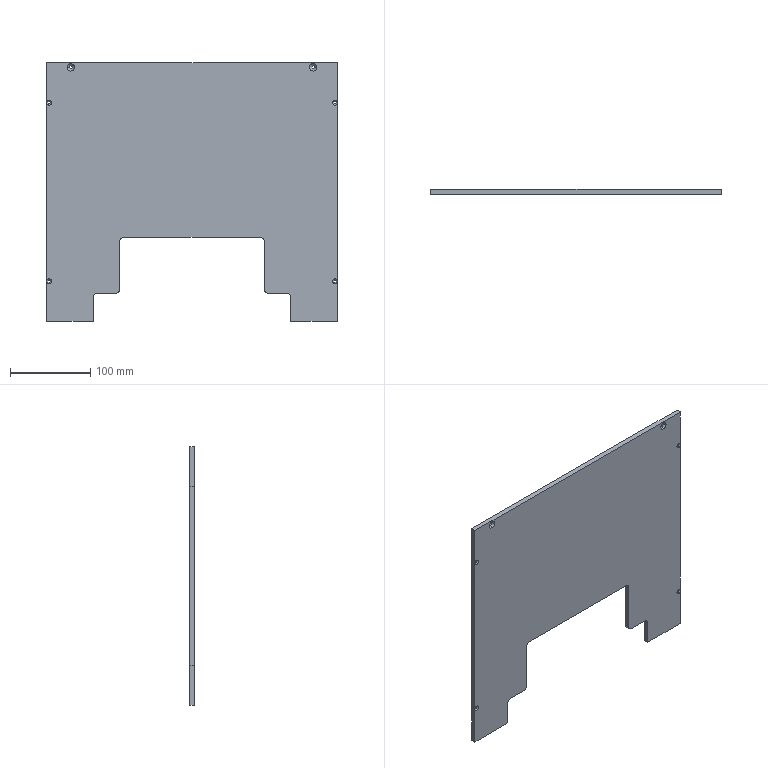Part | SolidWorks | features BaseBody 1 | 1 solid | 57 faces | box 362 x 6 x 322.5 mm | volume 572741 mm3 | cylinder 24 | cone 19 | plane 14 | commonest cylinder face diameters 3.2 x12 4.2 x6 10 x6